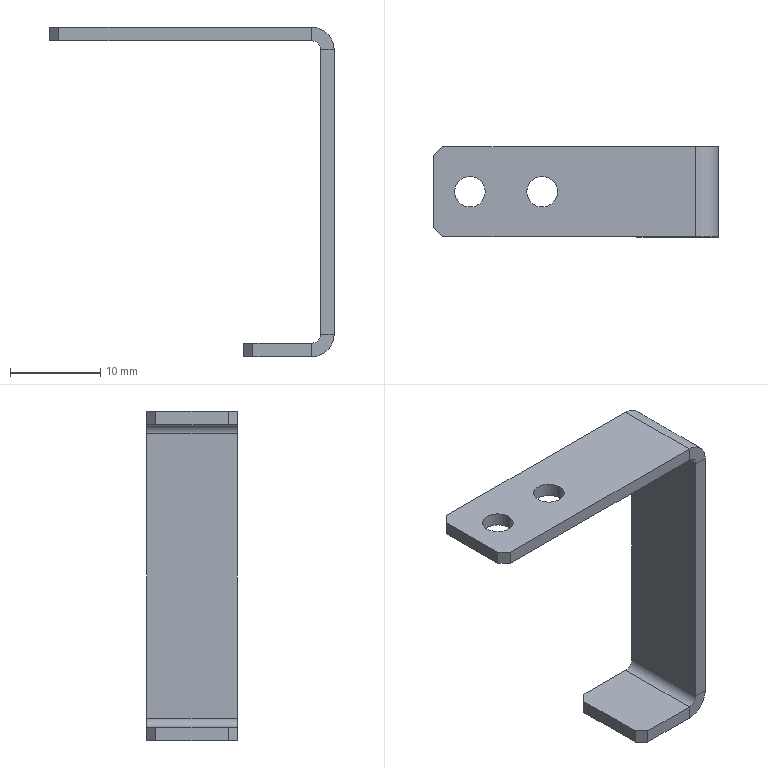Part | STEP file | FBDS-CS-005 | 1 solid | 30 faces | box 31.5 x 10 x 36.5 mm | volume 1072 mm3 | plane 22 | cylinder 8 | commonest cylinder face diameters 3.4 x4 2 x2 5 x2
STEP:
#1=CARTESIAN_POINT('',(-9.3,0.,-1.5));
#2=VERTEX_POINT('',#1);
#3=CARTESIAN_POINT('',(-12.7,0.,-1.5));
#4=VERTEX_POINT('',#3);
#5=CARTESIAN_POINT('',(-11.,0.,-1.5));
#6=DIRECTION('',(0.,0.,-1.));
#7=DIRECTION('',(-1.,0.,0.));
#8=AXIS2_PLACEMENT_3D('',#5,#6,#7);
#9=CIRCLE('',#8,1.7);
#10=EDGE_CURVE('',#2,#4,#9,.T.);
#11=ORIENTED_EDGE('',*,*,#10,.T.);
#12=CARTESIAN_POINT('',(-12.7,0.,0.));
#13=VERTEX_POINT('',#12);
#14=CARTESIAN_POINT('',(-12.7,0.,0.));
#15=DIRECTION('',(0.,0.,1.));
#16=VECTOR('',#15,1000.);
#17=LINE('',#14,#16);
#18=EDGE_CURVE('',#4,#13,#17,.T.);
#19=ORIENTED_EDGE('',*,*,#18,.T.);
#20=CARTESIAN_POINT('',(-9.3,0.,0.));
#21=VERTEX_POINT('',#20);
#22=CARTESIAN_POINT('',(-11.,0.,0.));
#23=DIRECTION('',(0.,0.,1.));
#24=DIRECTION('',(1.,0.,0.));
#25=AXIS2_PLACEMENT_3D('',#22,#23,#24);
#26=CIRCLE('',#25,1.7);
#27=EDGE_CURVE('',#13,#21,#26,.T.);
#28=ORIENTED_EDGE('',*,*,#27,.T.);
#29=CARTESIAN_POINT('',(-9.3,0.,0.));
#30=DIRECTION('',(0.,0.,1.));
#31=VECTOR('',#30,1000.);
#32=LINE('',#29,#31);
#33=EDGE_CURVE('',#2,#21,#32,.T.);
#34=ORIENTED_EDGE('',*,*,#33,.F.);
#35=EDGE_LOOP('',(#11,#19,#28,#34));
#36=FACE_OUTER_BOUND('',#35,.T.);
#37=CARTESIAN_POINT('',(-11.,0.,0.));
#38=DIRECTION('',(0.,0.,1.));
#39=DIRECTION('',(1.,0.,0.));
#40=AXIS2_PLACEMENT_3D('',#37,#38,#39);
#41=CYLINDRICAL_SURFACE('',#40,1.7);
#42=ADVANCED_FACE('',(#36),#41,.F.);
#43=CARTESIAN_POINT('',(-1.3,0.,-1.5));
#44=VERTEX_POINT('',#43);
#45=CARTESIAN_POINT('',(-4.7,0.,-1.5));
#46=VERTEX_POINT('',#45);
#47=CARTESIAN_POINT('',(-3.,0.,-1.5));
#48=DIRECTION('',(0.,0.,-1.));
#49=DIRECTION('',(-1.,0.,0.));
#50=AXIS2_PLACEMENT_3D('',#47,#48,#49);
#51=CIRCLE('',#50,1.7);
#52=EDGE_CURVE('',#44,#46,#51,.T.);
#53=ORIENTED_EDGE('',*,*,#52,.T.);
#54=CARTESIAN_POINT('',(-4.7,0.,0.));
#55=VERTEX_POINT('',#54);
#56=CARTESIAN_POINT('',(-4.7,0.,0.));
#57=DIRECTION('',(0.,0.,1.));
#58=VECTOR('',#57,1000.);
#59=LINE('',#56,#58);
#60=EDGE_CURVE('',#46,#55,#59,.T.);
#61=ORIENTED_EDGE('',*,*,#60,.T.);
#62=CARTESIAN_POINT('',(-1.3,0.,0.));
#63=VERTEX_POINT('',#62);
#64=CARTESIAN_POINT('',(-3.,0.,0.));
#65=DIRECTION('',(0.,0.,1.));
#66=DIRECTION('',(1.,0.,0.));
#67=AXIS2_PLACEMENT_3D('',#64,#65,#66);
#68=CIRCLE('',#67,1.7);
#69=EDGE_CURVE('',#55,#63,#68,.T.);
#70=ORIENTED_EDGE('',*,*,#69,.T.);
#71=CARTESIAN_POINT('',(-1.3,0.,0.));
#72=DIRECTION('',(0.,0.,1.));
#73=VECTOR('',#72,1000.);
#74=LINE('',#71,#73);
#75=EDGE_CURVE('',#44,#63,#74,.T.);
#76=ORIENTED_EDGE('',*,*,#75,.F.);
#77=EDGE_LOOP('',(#53,#61,#70,#76));
#78=FACE_OUTER_BOUND('',#77,.T.);
#79=CARTESIAN_POINT('',(-3.,0.,0.));
#80=DIRECTION('',(0.,0.,1.));
#81=DIRECTION('',(1.,0.,0.));
#82=AXIS2_PLACEMENT_3D('',#79,#80,#81);
#83=CYLINDRICAL_SURFACE('',#82,1.7);
#84=ADVANCED_FACE('',(#78),#83,.F.);
#85=CARTESIAN_POINT('',(15.,-5.,-34.));
#86=VERTEX_POINT('',#85);
#87=CARTESIAN_POINT('',(16.5,-5.,-34.));
#88=VERTEX_POINT('',#87);
#89=CARTESIAN_POINT('',(15.,-5.,-34.));
#90=DIRECTION('',(1.,0.,0.));
#91=VECTOR('',#90,1000.);
#92=LINE('',#89,#91);
#93=EDGE_CURVE('',#86,#88,#92,.T.);
#94=ORIENTED_EDGE('',*,*,#93,.T.);
#95=CARTESIAN_POINT('',(16.5,-5.,-2.5));
#96=VERTEX_POINT('',#95);
#97=CARTESIAN_POINT('',(16.5,-5.,-35.));
#98=DIRECTION('',(0.,0.,-1.));
#99=VECTOR('',#98,1000.);
#100=LINE('',#97,#99);
#101=EDGE_CURVE('',#96,#88,#100,.T.);
#102=ORIENTED_EDGE('',*,*,#101,.F.);
#103=CARTESIAN_POINT('',(15.,-5.,-2.5));
#104=VERTEX_POINT('',#103);
#105=CARTESIAN_POINT('',(15.,-5.,-2.5));
#106=DIRECTION('',(1.,0.,0.));
#107=VECTOR('',#106,1000.);
#108=LINE('',#105,#107);
#109=EDGE_CURVE('',#104,#96,#108,.T.);
#110=ORIENTED_EDGE('',*,*,#109,.F.);
#111=CARTESIAN_POINT('',(15.,-5.,-35.));
#112=DIRECTION('',(0.,0.,-1.));
#113=VECTOR('',#112,1000.);
#114=LINE('',#111,#113);
#115=EDGE_CURVE('',#104,#86,#114,.T.);
#116=ORIENTED_EDGE('',*,*,#115,.T.);
#117=EDGE_LOOP('',(#94,#102,#110,#116));
#118=FACE_OUTER_BOUND('',#117,.T.);
#119=CARTESIAN_POINT('',(16.5,-5.,-35.));
#120=DIRECTION('',(0.,1.,0.));
#121=DIRECTION('',(0.,0.,1.));
#122=AXIS2_PLACEMENT_3D('',#119,#120,#121);
#123=PLANE('',#122);
#124=ADVANCED_FACE('',(#118),#123,.F.);
#125=CARTESIAN_POINT('',(15.,5.,-34.));
#126=VERTEX_POINT('',#125);
#127=CARTESIAN_POINT('',(16.5,5.,-34.));
#128=VERTEX_POINT('',#127);
#129=CARTESIAN_POINT('',(15.,5.,-34.));
#130=DIRECTION('',(1.,0.,0.));
#131=VECTOR('',#130,1000.);
#132=LINE('',#129,#131);
#133=EDGE_CURVE('',#126,#128,#132,.T.);
#134=ORIENTED_EDGE('',*,*,#133,.F.);
#135=CARTESIAN_POINT('',(15.,5.,-2.5));
#136=VERTEX_POINT('',#135);
#137=CARTESIAN_POINT('',(15.,5.,-1.5));
#138=DIRECTION('',(0.,0.,1.));
#139=VECTOR('',#138,1000.);
#140=LINE('',#137,#139);
#141=EDGE_CURVE('',#126,#136,#140,.T.);
#142=ORIENTED_EDGE('',*,*,#141,.T.);
#143=CARTESIAN_POINT('',(16.5,5.,-2.5));
#144=VERTEX_POINT('',#143);
#145=CARTESIAN_POINT('',(15.,5.,-2.5));
#146=DIRECTION('',(1.,0.,0.));
#147=VECTOR('',#146,1000.);
#148=LINE('',#145,#147);
#149=EDGE_CURVE('',#136,#144,#148,.T.);
#150=ORIENTED_EDGE('',*,*,#149,.T.);
#151=CARTESIAN_POINT('',(16.5,5.,-1.5));
#152=DIRECTION('',(0.,0.,1.));
#153=VECTOR('',#152,1000.);
#154=LINE('',#151,#153);
#155=EDGE_CURVE('',#128,#144,#154,.T.);
#156=ORIENTED_EDGE('',*,*,#155,.F.);
#157=EDGE_LOOP('',(#134,#142,#150,#156));
#158=FACE_OUTER_BOUND('',#157,.T.);
#159=CARTESIAN_POINT('',(16.5,5.,-1.5));
#160=DIRECTION('',(0.,-1.,0.));
#161=DIRECTION('',(0.,0.,-1.));
#162=AXIS2_PLACEMENT_3D('',#159,#160,#161);
#163=PLANE('',#162);
#164=ADVANCED_FACE('',(#158),#163,.F.);
#165=CARTESIAN_POINT('',(16.5,-5.,-34.));
#166=DIRECTION('',(0.,1.,0.));
#167=VECTOR('',#166,1000.);
#168=LINE('',#165,#167);
#169=EDGE_CURVE('',#88,#128,#168,.T.);
#170=ORIENTED_EDGE('',*,*,#169,.T.);
#171=ORIENTED_EDGE('',*,*,#155,.T.);
#172=CARTESIAN_POINT('',(16.5,0.,-2.5));
#173=DIRECTION('',(0.,1.,0.));
#174=VECTOR('',#173,1000.);
#175=LINE('',#172,#174);
#176=EDGE_CURVE('',#96,#144,#175,.T.);
#177=ORIENTED_EDGE('',*,*,#176,.F.);
#178=ORIENTED_EDGE('',*,*,#101,.T.);
#179=EDGE_LOOP('',(#170,#171,#177,#178));
#180=FACE_OUTER_BOUND('',#179,.T.);
#181=CARTESIAN_POINT('',(16.5,0.,0.));
#182=DIRECTION('',(-1.,0.,0.));
#183=DIRECTION('',(0.,0.,1.));
#184=AXIS2_PLACEMENT_3D('',#181,#182,#183);
#185=PLANE('',#184);
#186=ADVANCED_FACE('',(#180),#185,.F.);
#187=ORIENTED_EDGE('',*,*,#141,.F.);
#188=CARTESIAN_POINT('',(15.,-5.,-34.));
#189=DIRECTION('',(0.,1.,0.));
#190=VECTOR('',#189,1000.);
#191=LINE('',#188,#190);
#192=EDGE_CURVE('',#86,#126,#191,.T.);
#193=ORIENTED_EDGE('',*,*,#192,.F.);
#194=ORIENTED_EDGE('',*,*,#115,.F.);
#195=CARTESIAN_POINT('',(15.,5.,-2.5));
#196=DIRECTION('',(0.,-1.,0.));
#197=VECTOR('',#196,1000.);
#198=LINE('',#195,#197);
#199=EDGE_CURVE('',#136,#104,#198,.T.);
#200=ORIENTED_EDGE('',*,*,#199,.F.);
#201=EDGE_LOOP('',(#187,#193,#194,#200));
#202=FACE_OUTER_BOUND('',#201,.T.);
#203=CARTESIAN_POINT('',(15.,0.,0.));
#204=DIRECTION('',(-1.,0.,0.));
#205=DIRECTION('',(0.,0.,1.));
#206=AXIS2_PLACEMENT_3D('',#203,#204,#205);
#207=PLANE('',#206);
#208=ADVANCED_FACE('',(#202),#207,.T.);
#209=CARTESIAN_POINT('',(-14.,-5.,0.));
#210=VERTEX_POINT('',#209);
#211=CARTESIAN_POINT('',(14.,-5.,0.));
#212=VERTEX_POINT('',#211);
#213=CARTESIAN_POINT('',(-15.,-5.,0.));
#214=DIRECTION('',(1.,0.,0.));
#215=VECTOR('',#214,1000.);
#216=LINE('',#213,#215);
#217=EDGE_CURVE('',#210,#212,#216,.T.);
#218=ORIENTED_EDGE('',*,*,#217,.F.);
#219=CARTESIAN_POINT('',(-14.,-5.,-1.5));
#220=VERTEX_POINT('',#219);
#221=CARTESIAN_POINT('',(-14.,-5.,-1.5));
#222=DIRECTION('',(0.,0.,-1.));
#223=VECTOR('',#222,1000.);
#224=LINE('',#221,#223);
#225=EDGE_CURVE('',#210,#220,#224,.T.);
#226=ORIENTED_EDGE('',*,*,#225,.T.);
#227=CARTESIAN_POINT('',(14.,-5.,-1.5));
#228=VERTEX_POINT('',#227);
#229=CARTESIAN_POINT('',(-15.,-5.,-1.5));
#230=DIRECTION('',(1.,0.,0.));
#231=VECTOR('',#230,1000.);
#232=LINE('',#229,#231);
#233=EDGE_CURVE('',#220,#228,#232,.T.);
#234=ORIENTED_EDGE('',*,*,#233,.T.);
#235=CARTESIAN_POINT('',(14.,-5.,-1.5));
#236=DIRECTION('',(0.,0.,1.));
#237=VECTOR('',#236,1000.);
#238=LINE('',#235,#237);
#239=EDGE_CURVE('',#228,#212,#238,.T.);
#240=ORIENTED_EDGE('',*,*,#239,.T.);
#241=EDGE_LOOP('',(#218,#226,#234,#240));
#242=FACE_OUTER_BOUND('',#241,.T.);
#243=CARTESIAN_POINT('',(-15.,-5.,-1.5));
#244=DIRECTION('',(0.,-1.,0.));
#245=DIRECTION('',(0.,0.,-1.));
#246=AXIS2_PLACEMENT_3D('',#243,#244,#245);
#247=PLANE('',#246);
#248=ADVANCED_FACE('',(#242),#247,.T.);
#249=ORIENTED_EDGE('',*,*,#10,.F.);
#250=CARTESIAN_POINT('',(-11.,0.,-1.5));
#251=DIRECTION('',(0.,0.,-1.));
#252=DIRECTION('',(-1.,0.,0.));
#253=AXIS2_PLACEMENT_3D('',#250,#251,#252);
#254=CIRCLE('',#253,1.7);
#255=EDGE_CURVE('',#4,#2,#254,.T.);
#256=ORIENTED_EDGE('',*,*,#255,.F.);
#257=EDGE_LOOP('',(#249,#256));
#258=FACE_BOUND('',#257,.T.);
#259=ORIENTED_EDGE('',*,*,#52,.F.);
#260=CARTESIAN_POINT('',(-3.,0.,-1.5));
#261=DIRECTION('',(0.,0.,-1.));
#262=DIRECTION('',(-1.,0.,0.));
#263=AXIS2_PLACEMENT_3D('',#260,#261,#262);
#264=CIRCLE('',#263,1.7);
#265=EDGE_CURVE('',#46,#44,#264,.T.);
#266=ORIENTED_EDGE('',*,*,#265,.F.);
#267=EDGE_LOOP('',(#259,#266));
#268=FACE_BOUND('',#267,.T.);
#269=CARTESIAN_POINT('',(-15.,4.,-1.5));
#270=VERTEX_POINT('',#269);
#271=CARTESIAN_POINT('',(-15.,-4.,-1.5));
#272=VERTEX_POINT('',#271);
#273=CARTESIAN_POINT('',(-15.,-5.,-1.5));
#274=DIRECTION('',(0.,-1.,0.));
#275=VECTOR('',#274,1000.);
#276=LINE('',#273,#275);
#277=EDGE_CURVE('',#270,#272,#276,.T.);
#278=ORIENTED_EDGE('',*,*,#277,.F.);
#279=CARTESIAN_POINT('',(-14.,5.,-1.5));
#280=VERTEX_POINT('',#279);
#281=CARTESIAN_POINT('',(-9.5,9.5,-1.5));
#282=DIRECTION('',(0.7071,0.7071,0.));
#283=VECTOR('',#282,1000.);
#284=LINE('',#281,#283);
#285=EDGE_CURVE('',#270,#280,#284,.T.);
#286=ORIENTED_EDGE('',*,*,#285,.T.);
#287=CARTESIAN_POINT('',(14.,5.,-1.5));
#288=VERTEX_POINT('',#287);
#289=CARTESIAN_POINT('',(-15.,5.,-1.5));
#290=DIRECTION('',(-1.,0.,0.));
#291=VECTOR('',#290,1000.);
#292=LINE('',#289,#291);
#293=EDGE_CURVE('',#288,#280,#292,.T.);
#294=ORIENTED_EDGE('',*,*,#293,.F.);
#295=CARTESIAN_POINT('',(14.,-5.,-1.5));
#296=DIRECTION('',(0.,1.,0.));
#297=VECTOR('',#296,1000.);
#298=LINE('',#295,#297);
#299=EDGE_CURVE('',#228,#288,#298,.T.);
#300=ORIENTED_EDGE('',*,*,#299,.F.);
#301=ORIENTED_EDGE('',*,*,#233,.F.);
#302=CARTESIAN_POINT('',(-9.5,-9.5,-1.5));
#303=DIRECTION('',(-0.7071,0.7071,0.));
#304=VECTOR('',#303,1000.);
#305=LINE('',#302,#304);
#306=EDGE_CURVE('',#220,#272,#305,.T.);
#307=ORIENTED_EDGE('',*,*,#306,.T.);
#308=EDGE_LOOP('',(#278,#286,#294,#300,#301,#307));
#309=FACE_OUTER_BOUND('',#308,.T.);
#310=CARTESIAN_POINT('',(0.,0.,-1.5));
#311=DIRECTION('',(0.,0.,-1.));
#312=DIRECTION('',(-1.,0.,0.));
#313=AXIS2_PLACEMENT_3D('',#310,#311,#312);
#314=PLANE('',#313);
#315=ADVANCED_FACE('',(#258,#268,#309),#314,.T.);
#316=CARTESIAN_POINT('',(-11.,0.,0.));
#317=DIRECTION('',(0.,0.,1.));
#318=DIRECTION('',(1.,0.,0.));
#319=AXIS2_PLACEMENT_3D('',#316,#317,#318);
#320=CIRCLE('',#319,1.7);
#321=EDGE_CURVE('',#21,#13,#320,.T.);
#322=ORIENTED_EDGE('',*,*,#321,.F.);
#323=ORIENTED_EDGE('',*,*,#27,.F.);
#324=EDGE_LOOP('',(#322,#323));
#325=FACE_BOUND('',#324,.T.);
#326=CARTESIAN_POINT('',(-3.,0.,0.));
#327=DIRECTION('',(0.,0.,1.));
#328=DIRECTION('',(1.,0.,0.));
#329=AXIS2_PLACEMENT_3D('',#326,#327,#328);
#330=CIRCLE('',#329,1.7);
#331=EDGE_CURVE('',#63,#55,#330,.T.);
#332=ORIENTED_EDGE('',*,*,#331,.F.);
#333=ORIENTED_EDGE('',*,*,#69,.F.);
#334=EDGE_LOOP('',(#332,#333));
#335=FACE_BOUND('',#334,.T.);
#336=CARTESIAN_POINT('',(14.,5.,0.));
#337=VERTEX_POINT('',#336);
#338=CARTESIAN_POINT('',(-14.,5.,0.));
#339=VERTEX_POINT('',#338);
#340=CARTESIAN_POINT('',(-15.,5.,0.));
#341=DIRECTION('',(-1.,0.,0.));
#342=VECTOR('',#341,1000.);
#343=LINE('',#340,#342);
#344=EDGE_CURVE('',#337,#339,#343,.T.);
#345=ORIENTED_EDGE('',*,*,#344,.T.);
#346=CARTESIAN_POINT('',(-15.,4.,0.));
#347=VERTEX_POINT('',#346);
#348=CARTESIAN_POINT('',(-14.,5.,0.));
#349=DIRECTION('',(-0.7071,-0.7071,0.));
#350=VECTOR('',#349,1000.);
#351=LINE('',#348,#350);
#352=EDGE_CURVE('',#339,#347,#351,.T.);
#353=ORIENTED_EDGE('',*,*,#352,.T.);
#354=CARTESIAN_POINT('',(-15.,-4.,0.));
#355=VERTEX_POINT('',#354);
#356=CARTESIAN_POINT('',(-15.,-5.,0.));
#357=DIRECTION('',(0.,-1.,0.));
#358=VECTOR('',#357,1000.);
#359=LINE('',#356,#358);
#360=EDGE_CURVE('',#347,#355,#359,.T.);
#361=ORIENTED_EDGE('',*,*,#360,.T.);
#362=CARTESIAN_POINT('',(-15.,-4.,0.));
#363=DIRECTION('',(0.7071,-0.7071,0.));
#364=VECTOR('',#363,1000.);
#365=LINE('',#362,#364);
#366=EDGE_CURVE('',#355,#210,#365,.T.);
#367=ORIENTED_EDGE('',*,*,#366,.T.);
#368=ORIENTED_EDGE('',*,*,#217,.T.);
#369=CARTESIAN_POINT('',(14.,-5.,0.));
#370=DIRECTION('',(0.,1.,0.));
#371=VECTOR('',#370,1000.);
#372=LINE('',#369,#371);
#373=EDGE_CURVE('',#212,#337,#372,.T.);
#374=ORIENTED_EDGE('',*,*,#373,.T.);
#375=EDGE_LOOP('',(#345,#353,#361,#367,#368,#374));
#376=FACE_OUTER_BOUND('',#375,.T.);
#377=CARTESIAN_POINT('',(0.,0.,0.));
#378=DIRECTION('',(0.,0.,-1.));
#379=DIRECTION('',(-1.,0.,0.));
#380=AXIS2_PLACEMENT_3D('',#377,#378,#379);
#381=PLANE('',#380);
#382=ADVANCED_FACE('',(#325,#335,#376),#381,.F.);
#383=ORIENTED_EDGE('',*,*,#360,.F.);
#384=CARTESIAN_POINT('',(-15.,4.,-1.5));
#385=DIRECTION('',(0.,0.,-1.));
#386=VECTOR('',#385,1000.);
#387=LINE('',#384,#386);
#388=EDGE_CURVE('',#347,#270,#387,.T.);
#389=ORIENTED_EDGE('',*,*,#388,.T.);
#390=ORIENTED_EDGE('',*,*,#277,.T.);
#391=CARTESIAN_POINT('',(-15.,-4.,-1.5));
#392=DIRECTION('',(0.,0.,1.));
#393=VECTOR('',#392,1000.);
#394=LINE('',#391,#393);
#395=EDGE_CURVE('',#272,#355,#394,.T.);
#396=ORIENTED_EDGE('',*,*,#395,.T.);
#397=EDGE_LOOP('',(#383,#389,#390,#396));
#398=FACE_OUTER_BOUND('',#397,.T.);
#399=CARTESIAN_POINT('',(-15.,-5.,-1.5));
#400=DIRECTION('',(-1.,0.,0.));
#401=DIRECTION('',(0.,0.,1.));
#402=AXIS2_PLACEMENT_3D('',#399,#400,#401);
#403=PLANE('',#402);
#404=ADVANCED_FACE('',(#398),#403,.T.);
#405=ORIENTED_EDGE('',*,*,#293,.T.);
#406=CARTESIAN_POINT('',(-14.,5.,-1.5));
#407=DIRECTION('',(0.,0.,1.));
#408=VECTOR('',#407,1000.);
#409=LINE('',#406,#408);
#410=EDGE_CURVE('',#280,#339,#409,.T.);
#411=ORIENTED_EDGE('',*,*,#410,.T.);
#412=ORIENTED_EDGE('',*,*,#344,.F.);
#413=CARTESIAN_POINT('',(14.,5.,-1.5));
#414=DIRECTION('',(0.,0.,1.));
#415=VECTOR('',#414,1000.);
#416=LINE('',#413,#415);
#417=EDGE_CURVE('',#288,#337,#416,.T.);
#418=ORIENTED_EDGE('',*,*,#417,.F.);
#419=EDGE_LOOP('',(#405,#411,#412,#418));
#420=FACE_OUTER_BOUND('',#419,.T.);
#421=CARTESIAN_POINT('',(-15.,5.,-1.5));
#422=DIRECTION('',(0.,1.,0.));
#423=DIRECTION('',(0.,0.,1.));
#424=AXIS2_PLACEMENT_3D('',#421,#422,#423);
#425=PLANE('',#424);
#426=ADVANCED_FACE('',(#420),#425,.T.);
#427=ORIENTED_EDGE('',*,*,#149,.F.);
#428=CARTESIAN_POINT('',(14.,5.,-2.5));
#429=DIRECTION('',(0.,1.,0.));
#430=DIRECTION('',(0.,0.,-1.));
#431=AXIS2_PLACEMENT_3D('',#428,#429,#430);
#432=CIRCLE('',#431,1.);
#433=EDGE_CURVE('',#288,#136,#432,.T.);
#434=ORIENTED_EDGE('',*,*,#433,.F.);
#435=ORIENTED_EDGE('',*,*,#417,.T.);
#436=CARTESIAN_POINT('',(14.,5.,-2.5));
#437=DIRECTION('',(0.,1.,0.));
#438=DIRECTION('',(0.,0.,-1.));
#439=AXIS2_PLACEMENT_3D('',#436,#437,#438);
#440=CIRCLE('',#439,2.5);
#441=EDGE_CURVE('',#337,#144,#440,.T.);
#442=ORIENTED_EDGE('',*,*,#441,.T.);
#443=EDGE_LOOP('',(#427,#434,#435,#442));
#444=FACE_OUTER_BOUND('',#443,.T.);
#445=CARTESIAN_POINT('',(14.,5.,-2.5));
#446=DIRECTION('',(0.,1.,0.));
#447=DIRECTION('',(0.,0.,1.));
#448=AXIS2_PLACEMENT_3D('',#445,#446,#447);
#449=PLANE('',#448);
#450=ADVANCED_FACE('',(#444),#449,.T.);
#451=CARTESIAN_POINT('',(14.,-5.,-2.5));
#452=DIRECTION('',(0.,-1.,0.));
#453=DIRECTION('',(0.,0.,-1.));
#454=AXIS2_PLACEMENT_3D('',#451,#452,#453);
#455=CIRCLE('',#454,1.);
#456=EDGE_CURVE('',#104,#228,#455,.T.);
#457=ORIENTED_EDGE('',*,*,#456,.F.);
#458=ORIENTED_EDGE('',*,*,#109,.T.);
#459=CARTESIAN_POINT('',(14.,-5.,-2.5));
#460=DIRECTION('',(0.,-1.,0.));
#461=DIRECTION('',(0.,0.,-1.));
#462=AXIS2_PLACEMENT_3D('',#459,#460,#461);
#463=CIRCLE('',#462,2.5);
#464=EDGE_CURVE('',#96,#212,#463,.T.);
#465=ORIENTED_EDGE('',*,*,#464,.T.);
#466=ORIENTED_EDGE('',*,*,#239,.F.);
#467=EDGE_LOOP('',(#457,#458,#465,#466));
#468=FACE_OUTER_BOUND('',#467,.T.);
#469=CARTESIAN_POINT('',(14.,-5.,-2.5));
#470=DIRECTION('',(0.,1.,0.));
#471=DIRECTION('',(0.,0.,1.));
#472=AXIS2_PLACEMENT_3D('',#469,#470,#471);
#473=PLANE('',#472);
#474=ADVANCED_FACE('',(#468),#473,.F.);
#475=ORIENTED_EDGE('',*,*,#373,.F.);
#476=ORIENTED_EDGE('',*,*,#464,.F.);
#477=ORIENTED_EDGE('',*,*,#176,.T.);
#478=ORIENTED_EDGE('',*,*,#441,.F.);
#479=EDGE_LOOP('',(#475,#476,#477,#478));
#480=FACE_OUTER_BOUND('',#479,.T.);
#481=CARTESIAN_POINT('',(14.,-5.,-2.5));
#482=DIRECTION('',(0.,-1.,0.));
#483=DIRECTION('',(1.,0.,0.));
#484=AXIS2_PLACEMENT_3D('',#481,#482,#483);
#485=CYLINDRICAL_SURFACE('',#484,2.5);
#486=ADVANCED_FACE('',(#480),#485,.T.);
#487=ORIENTED_EDGE('',*,*,#299,.T.);
#488=ORIENTED_EDGE('',*,*,#433,.T.);
#489=ORIENTED_EDGE('',*,*,#199,.T.);
#490=ORIENTED_EDGE('',*,*,#456,.T.);
#491=EDGE_LOOP('',(#487,#488,#489,#490));
#492=FACE_OUTER_BOUND('',#491,.T.);
#493=CARTESIAN_POINT('',(14.,-5.,-2.5));
#494=DIRECTION('',(0.,-1.,0.));
#495=DIRECTION('',(1.,0.,0.));
#496=AXIS2_PLACEMENT_3D('',#493,#494,#495);
#497=CYLINDRICAL_SURFACE('',#496,1.);
#498=ADVANCED_FACE('',(#492),#497,.F.);
#499=CARTESIAN_POINT('',(14.,5.,-35.));
#500=VERTEX_POINT('',#499);
#501=CARTESIAN_POINT('',(14.,5.,-36.5));
#502=VERTEX_POINT('',#501);
#503=CARTESIAN_POINT('',(14.,5.,-35.));
#504=DIRECTION('',(0.,0.,-1.));
#505=VECTOR('',#504,1000.);
#506=LINE('',#503,#505);
#507=EDGE_CURVE('',#500,#502,#506,.T.);
#508=ORIENTED_EDGE('',*,*,#507,.F.);
#509=CARTESIAN_POINT('',(14.,5.,-34.));
#510=DIRECTION('',(0.,1.,0.));
#511=DIRECTION('',(0.,0.,-1.));
#512=AXIS2_PLACEMENT_3D('',#509,#510,#511);
#513=CIRCLE('',#512,1.);
#514=EDGE_CURVE('',#126,#500,#513,.T.);
#515=ORIENTED_EDGE('',*,*,#514,.F.);
#516=ORIENTED_EDGE('',*,*,#133,.T.);
#517=CARTESIAN_POINT('',(14.,5.,-34.));
#518=DIRECTION('',(0.,1.,0.));
#519=DIRECTION('',(0.,0.,-1.));
#520=AXIS2_PLACEMENT_3D('',#517,#518,#519);
#521=CIRCLE('',#520,2.5);
#522=EDGE_CURVE('',#128,#502,#521,.T.);
#523=ORIENTED_EDGE('',*,*,#522,.T.);
#524=EDGE_LOOP('',(#508,#515,#516,#523));
#525=FACE_OUTER_BOUND('',#524,.T.);
#526=CARTESIAN_POINT('',(14.,5.,-34.));
#527=DIRECTION('',(0.,1.,0.));
#528=DIRECTION('',(0.,0.,1.));
#529=AXIS2_PLACEMENT_3D('',#526,#527,#528);
#530=PLANE('',#529);
#531=ADVANCED_FACE('',(#525),#530,.T.);
#532=CARTESIAN_POINT('',(14.,-5.,-35.));
#533=VERTEX_POINT('',#532);
#534=CARTESIAN_POINT('',(14.,-5.,-34.));
#535=DIRECTION('',(0.,-1.,0.));
#536=DIRECTION('',(0.,0.,-1.));
#537=AXIS2_PLACEMENT_3D('',#534,#535,#536);
#538=CIRCLE('',#537,1.);
#539=EDGE_CURVE('',#533,#86,#538,.T.);
#540=ORIENTED_EDGE('',*,*,#539,.F.);
#541=CARTESIAN_POINT('',(14.,-5.,-36.5));
#542=VERTEX_POINT('',#541);
#543=CARTESIAN_POINT('',(14.,-5.,-35.));
#544=DIRECTION('',(0.,0.,-1.));
#545=VECTOR('',#544,1000.);
#546=LINE('',#543,#545);
#547=EDGE_CURVE('',#533,#542,#546,.T.);
#548=ORIENTED_EDGE('',*,*,#547,.T.);
#549=CARTESIAN_POINT('',(14.,-5.,-34.));
#550=DIRECTION('',(0.,-1.,0.));
#551=DIRECTION('',(0.,0.,-1.));
#552=AXIS2_PLACEMENT_3D('',#549,#550,#551);
#553=CIRCLE('',#552,2.5);
#554=EDGE_CURVE('',#542,#88,#553,.T.);
#555=ORIENTED_EDGE('',*,*,#554,.T.);
#556=ORIENTED_EDGE('',*,*,#93,.F.);
#557=EDGE_LOOP('',(#540,#548,#555,#556));
#558=FACE_OUTER_BOUND('',#557,.T.);
#559=CARTESIAN_POINT('',(14.,-5.,-34.));
#560=DIRECTION('',(0.,1.,0.));
#561=DIRECTION('',(0.,0.,1.));
#562=AXIS2_PLACEMENT_3D('',#559,#560,#561);
#563=PLANE('',#562);
#564=ADVANCED_FACE('',(#558),#563,.F.);
#565=ORIENTED_EDGE('',*,*,#169,.F.);
#566=ORIENTED_EDGE('',*,*,#554,.F.);
#567=CARTESIAN_POINT('',(14.,0.,-36.5));
#568=DIRECTION('',(0.,1.,0.));
#569=VECTOR('',#568,1000.);
#570=LINE('',#567,#569);
#571=EDGE_CURVE('',#542,#502,#570,.T.);
#572=ORIENTED_EDGE('',*,*,#571,.T.);
#573=ORIENTED_EDGE('',*,*,#522,.F.);
#574=EDGE_LOOP('',(#565,#566,#572,#573));
#575=FACE_OUTER_BOUND('',#574,.T.);
#576=CARTESIAN_POINT('',(14.,-5.,-34.));
#577=DIRECTION('',(0.,-1.,0.));
#578=DIRECTION('',(0.,0.,-1.));
#579=AXIS2_PLACEMENT_3D('',#576,#577,#578);
#580=CYLINDRICAL_SURFACE('',#579,2.5);
#581=ADVANCED_FACE('',(#575),#580,.T.);
#582=ORIENTED_EDGE('',*,*,#192,.T.);
#583=ORIENTED_EDGE('',*,*,#514,.T.);
#584=CARTESIAN_POINT('',(14.,5.,-35.));
#585=DIRECTION('',(0.,-1.,0.));
#586=VECTOR('',#585,1000.);
#587=LINE('',#584,#586);
#588=EDGE_CURVE('',#500,#533,#587,.T.);
#589=ORIENTED_EDGE('',*,*,#588,.T.);
#590=ORIENTED_EDGE('',*,*,#539,.T.);
#591=EDGE_LOOP('',(#582,#583,#589,#590));
#592=FACE_OUTER_BOUND('',#591,.T.);
#593=CARTESIAN_POINT('',(14.,-5.,-34.));
#594=DIRECTION('',(0.,-1.,0.));
#595=DIRECTION('',(0.,0.,-1.));
#596=AXIS2_PLACEMENT_3D('',#593,#594,#595);
#597=CYLINDRICAL_SURFACE('',#596,1.);
#598=ADVANCED_FACE('',(#592),#597,.F.);
#599=CARTESIAN_POINT('',(7.5,-5.,-35.));
#600=VERTEX_POINT('',#599);
#601=CARTESIAN_POINT('',(6.5,-5.,-35.));
#602=DIRECTION('',(-1.,0.,0.));
#603=VECTOR('',#602,1000.);
#604=LINE('',#601,#603);
#605=EDGE_CURVE('',#533,#600,#604,.T.);
#606=ORIENTED_EDGE('',*,*,#605,.T.);
#607=CARTESIAN_POINT('',(7.5,-5.,-36.5));
#608=VERTEX_POINT('',#607);
#609=CARTESIAN_POINT('',(7.5,-5.,-36.5));
#610=DIRECTION('',(0.,0.,-1.));
#611=VECTOR('',#610,1000.);
#612=LINE('',#609,#611);
#613=EDGE_CURVE('',#600,#608,#612,.T.);
#614=ORIENTED_EDGE('',*,*,#613,.T.);
#615=CARTESIAN_POINT('',(6.5,-5.,-36.5));
#616=DIRECTION('',(-1.,0.,0.));
#617=VECTOR('',#616,1000.);
#618=LINE('',#615,#617);
#619=EDGE_CURVE('',#542,#608,#618,.T.);
#620=ORIENTED_EDGE('',*,*,#619,.F.);
#621=ORIENTED_EDGE('',*,*,#547,.F.);
#622=EDGE_LOOP('',(#606,#614,#620,#621));
#623=FACE_OUTER_BOUND('',#622,.T.);
#624=CARTESIAN_POINT('',(6.5,-5.,-36.5));
#625=DIRECTION('',(0.,1.,0.));
#626=DIRECTION('',(0.,0.,1.));
#627=AXIS2_PLACEMENT_3D('',#624,#625,#626);
#628=PLANE('',#627);
#629=ADVANCED_FACE('',(#623),#628,.F.);
#630=CARTESIAN_POINT('',(7.5,5.,-36.5));
#631=VERTEX_POINT('',#630);
#632=CARTESIAN_POINT('',(15.,5.,-36.5));
#633=DIRECTION('',(1.,0.,0.));
#634=VECTOR('',#633,1000.);
#635=LINE('',#632,#634);
#636=EDGE_CURVE('',#631,#502,#635,.T.);
#637=ORIENTED_EDGE('',*,*,#636,.F.);
#638=CARTESIAN_POINT('',(7.5,5.,-35.));
#639=VERTEX_POINT('',#638);
#640=CARTESIAN_POINT('',(7.5,5.,-36.5));
#641=DIRECTION('',(0.,0.,1.));
#642=VECTOR('',#641,1000.);
#643=LINE('',#640,#642);
#644=EDGE_CURVE('',#631,#639,#643,.T.);
#645=ORIENTED_EDGE('',*,*,#644,.T.);
#646=CARTESIAN_POINT('',(15.,5.,-35.));
#647=DIRECTION('',(1.,0.,0.));
#648=VECTOR('',#647,1000.);
#649=LINE('',#646,#648);
#650=EDGE_CURVE('',#639,#500,#649,.T.);
#651=ORIENTED_EDGE('',*,*,#650,.T.);
#652=ORIENTED_EDGE('',*,*,#507,.T.);
#653=EDGE_LOOP('',(#637,#645,#651,#652));
#654=FACE_OUTER_BOUND('',#653,.T.);
#655=CARTESIAN_POINT('',(15.,5.,-36.5));
#656=DIRECTION('',(0.,-1.,0.));
#657=DIRECTION('',(0.,0.,-1.));
#658=AXIS2_PLACEMENT_3D('',#655,#656,#657);
#659=PLANE('',#658);
#660=ADVANCED_FACE('',(#654),#659,.F.);
#661=ORIENTED_EDGE('',*,*,#619,.T.);
#662=CARTESIAN_POINT('',(6.5,-4.,-36.5));
#663=VERTEX_POINT('',#662);
#664=CARTESIAN_POINT('',(6.5,-4.,-36.5));
#665=DIRECTION('',(-0.7071,0.7071,0.));
#666=VECTOR('',#665,1000.);
#667=LINE('',#664,#666);
#668=EDGE_CURVE('',#608,#663,#667,.T.);
#669=ORIENTED_EDGE('',*,*,#668,.T.);
#670=CARTESIAN_POINT('',(6.5,4.,-36.5));
#671=VERTEX_POINT('',#670);
#672=CARTESIAN_POINT('',(6.5,5.,-36.5));
#673=DIRECTION('',(0.,1.,0.));
#674=VECTOR('',#673,1000.);
#675=LINE('',#672,#674);
#676=EDGE_CURVE('',#663,#671,#675,.T.);
#677=ORIENTED_EDGE('',*,*,#676,.T.);
#678=CARTESIAN_POINT('',(7.5,5.,-36.5));
#679=DIRECTION('',(0.7071,0.7071,0.));
#680=VECTOR('',#679,1000.);
#681=LINE('',#678,#680);
#682=EDGE_CURVE('',#671,#631,#681,.T.);
#683=ORIENTED_EDGE('',*,*,#682,.T.);
#684=ORIENTED_EDGE('',*,*,#636,.T.);
#685=ORIENTED_EDGE('',*,*,#571,.F.);
#686=EDGE_LOOP('',(#661,#669,#677,#683,#684,#685));
#687=FACE_OUTER_BOUND('',#686,.T.);
#688=CARTESIAN_POINT('',(0.,0.,-36.5));
#689=DIRECTION('',(0.,0.,1.));
#690=DIRECTION('',(1.,0.,0.));
#691=AXIS2_PLACEMENT_3D('',#688,#689,#690);
#692=PLANE('',#691);
#693=ADVANCED_FACE('',(#687),#692,.F.);
#694=CARTESIAN_POINT('',(6.5,-4.,-35.));
#695=VERTEX_POINT('',#694);
#696=CARTESIAN_POINT('',(6.5,4.,-35.));
#697=VERTEX_POINT('',#696);
#698=CARTESIAN_POINT('',(6.5,5.,-35.));
#699=DIRECTION('',(0.,1.,0.));
#700=VECTOR('',#699,1000.);
#701=LINE('',#698,#700);
#702=EDGE_CURVE('',#695,#697,#701,.T.);
#703=ORIENTED_EDGE('',*,*,#702,.F.);
#704=CARTESIAN_POINT('',(1.25,1.25,-35.));
#705=DIRECTION('',(0.7071,-0.7071,0.));
#706=VECTOR('',#705,1000.);
#707=LINE('',#704,#706);
#708=EDGE_CURVE('',#695,#600,#707,.T.);
#709=ORIENTED_EDGE('',*,*,#708,.T.);
#710=ORIENTED_EDGE('',*,*,#605,.F.);
#711=ORIENTED_EDGE('',*,*,#588,.F.);
#712=ORIENTED_EDGE('',*,*,#650,.F.);
#713=CARTESIAN_POINT('',(1.25,-1.25,-35.));
#714=DIRECTION('',(-0.7071,-0.7071,0.));
#715=VECTOR('',#714,1000.);
#716=LINE('',#713,#715);
#717=EDGE_CURVE('',#639,#697,#716,.T.);
#718=ORIENTED_EDGE('',*,*,#717,.T.);
#719=EDGE_LOOP('',(#703,#709,#710,#711,#712,#718));
#720=FACE_OUTER_BOUND('',#719,.T.);
#721=CARTESIAN_POINT('',(0.,0.,-35.));
#722=DIRECTION('',(0.,0.,1.));
#723=DIRECTION('',(1.,0.,0.));
#724=AXIS2_PLACEMENT_3D('',#721,#722,#723);
#725=PLANE('',#724);
#726=ADVANCED_FACE('',(#720),#725,.T.);
#727=ORIENTED_EDGE('',*,*,#676,.F.);
#728=CARTESIAN_POINT('',(6.5,-4.,-36.5));
#729=DIRECTION('',(0.,0.,1.));
#730=VECTOR('',#729,1000.);
#731=LINE('',#728,#730);
#732=EDGE_CURVE('',#663,#695,#731,.T.);
#733=ORIENTED_EDGE('',*,*,#732,.T.);
#734=ORIENTED_EDGE('',*,*,#702,.T.);
#735=CARTESIAN_POINT('',(6.5,4.,-36.5));
#736=DIRECTION('',(0.,0.,-1.));
#737=VECTOR('',#736,1000.);
#738=LINE('',#735,#737);
#739=EDGE_CURVE('',#697,#671,#738,.T.);
#740=ORIENTED_EDGE('',*,*,#739,.T.);
#741=EDGE_LOOP('',(#727,#733,#734,#740));
#742=FACE_OUTER_BOUND('',#741,.T.);
#743=CARTESIAN_POINT('',(6.5,5.,-36.5));
#744=DIRECTION('',(1.,0.,0.));
#745=DIRECTION('',(0.,0.,-1.));
#746=AXIS2_PLACEMENT_3D('',#743,#744,#745);
#747=PLANE('',#746);
#748=ADVANCED_FACE('',(#742),#747,.F.);
#749=ORIENTED_EDGE('',*,*,#60,.F.);
#750=ORIENTED_EDGE('',*,*,#265,.T.);
#751=ORIENTED_EDGE('',*,*,#75,.T.);
#752=ORIENTED_EDGE('',*,*,#331,.T.);
#753=EDGE_LOOP('',(#749,#750,#751,#752));
#754=FACE_OUTER_BOUND('',#753,.T.);
#755=CARTESIAN_POINT('',(-3.,0.,0.));
#756=DIRECTION('',(0.,0.,1.));
#757=DIRECTION('',(1.,0.,0.));
#758=AXIS2_PLACEMENT_3D('',#755,#756,#757);
#759=CYLINDRICAL_SURFACE('',#758,1.7);
#760=ADVANCED_FACE('',(#754),#759,.F.);
#761=ORIENTED_EDGE('',*,*,#18,.F.);
#762=ORIENTED_EDGE('',*,*,#255,.T.);
#763=ORIENTED_EDGE('',*,*,#33,.T.);
#764=ORIENTED_EDGE('',*,*,#321,.T.);
#765=EDGE_LOOP('',(#761,#762,#763,#764));
#766=FACE_OUTER_BOUND('',#765,.T.);
#767=CARTESIAN_POINT('',(-11.,0.,0.));
#768=DIRECTION('',(0.,0.,1.));
#769=DIRECTION('',(1.,0.,0.));
#770=AXIS2_PLACEMENT_3D('',#767,#768,#769);
#771=CYLINDRICAL_SURFACE('',#770,1.7);
#772=ADVANCED_FACE('',(#766),#771,.F.);
#773=ORIENTED_EDGE('',*,*,#668,.F.);
#774=ORIENTED_EDGE('',*,*,#613,.F.);
#775=ORIENTED_EDGE('',*,*,#708,.F.);
#776=ORIENTED_EDGE('',*,*,#732,.F.);
#777=EDGE_LOOP('',(#773,#774,#775,#776));
#778=FACE_OUTER_BOUND('',#777,.T.);
#779=CARTESIAN_POINT('',(6.5,-4.,-36.5));
#780=DIRECTION('',(0.7071,0.7071,0.));
#781=DIRECTION('',(0.,0.,1.));
#782=AXIS2_PLACEMENT_3D('',#779,#780,#781);
#783=PLANE('',#782);
#784=ADVANCED_FACE('',(#778),#783,.F.);
#785=ORIENTED_EDGE('',*,*,#682,.F.);
#786=ORIENTED_EDGE('',*,*,#739,.F.);
#787=ORIENTED_EDGE('',*,*,#717,.F.);
#788=ORIENTED_EDGE('',*,*,#644,.F.);
#789=EDGE_LOOP('',(#785,#786,#787,#788));
#790=FACE_OUTER_BOUND('',#789,.T.);
#791=CARTESIAN_POINT('',(7.5,5.,-36.5));
#792=DIRECTION('',(0.7071,-0.7071,0.));
#793=DIRECTION('',(0.,0.,1.));
#794=AXIS2_PLACEMENT_3D('',#791,#792,#793);
#795=PLANE('',#794);
#796=ADVANCED_FACE('',(#790),#795,.F.);
#797=ORIENTED_EDGE('',*,*,#285,.F.);
#798=ORIENTED_EDGE('',*,*,#388,.F.);
#799=ORIENTED_EDGE('',*,*,#352,.F.);
#800=ORIENTED_EDGE('',*,*,#410,.F.);
#801=EDGE_LOOP('',(#797,#798,#799,#800));
#802=FACE_OUTER_BOUND('',#801,.T.);
#803=CARTESIAN_POINT('',(-14.,5.,-1.5));
#804=DIRECTION('',(0.7071,-0.7071,0.));
#805=DIRECTION('',(0.,0.,1.));
#806=AXIS2_PLACEMENT_3D('',#803,#804,#805);
#807=PLANE('',#806);
#808=ADVANCED_FACE('',(#802),#807,.F.);
#809=ORIENTED_EDGE('',*,*,#306,.F.);
#810=ORIENTED_EDGE('',*,*,#225,.F.);
#811=ORIENTED_EDGE('',*,*,#366,.F.);
#812=ORIENTED_EDGE('',*,*,#395,.F.);
#813=EDGE_LOOP('',(#809,#810,#811,#812));
#814=FACE_OUTER_BOUND('',#813,.T.);
#815=CARTESIAN_POINT('',(-15.,-4.,-1.5));
#816=DIRECTION('',(0.7071,0.7071,0.));
#817=DIRECTION('',(0.,0.,1.));
#818=AXIS2_PLACEMENT_3D('',#815,#816,#817);
#819=PLANE('',#818);
#820=ADVANCED_FACE('',(#814),#819,.F.);
#821=CLOSED_SHELL('',(#42,#84,#124,#164,#186,#208,#248,#315,#382,#404,#426,#450,#474,#486,#498,#531,#564,#581,#598,#629,#660,#693,#726,#748,#760,#772,#784,#796,#808,#820));
#822=MANIFOLD_SOLID_BREP('',#821);
#823=CARTESIAN_POINT('',(0.,0.,0.));
#824=DIRECTION('',(0.,0.,1.));
#825=DIRECTION('',(1.,0.,0.));
#826=AXIS2_PLACEMENT_3D('',#823,#824,#825);
#827=(LENGTH_UNIT()NAMED_UNIT(*)SI_UNIT(.MILLI.,.METRE.));
#828=UNCERTAINTY_MEASURE_WITH_UNIT(LENGTH_MEASURE(0.00001),#827,'','');
#829=(NAMED_UNIT(*)PLANE_ANGLE_UNIT()SI_UNIT($,.RADIAN.));
#830=(NAMED_UNIT(*)SI_UNIT($,.STERADIAN.)SOLID_ANGLE_UNIT());
#831=(GEOMETRIC_REPRESENTATION_CONTEXT(3)GLOBAL_UNCERTAINTY_ASSIGNED_CONTEXT((#828))GLOBAL_UNIT_ASSIGNED_CONTEXT((#827,#829,#830))REPRESENTATION_CONTEXT('',''));
#832=ADVANCED_BREP_SHAPE_REPRESENTATION('',(#822,#826),#831);